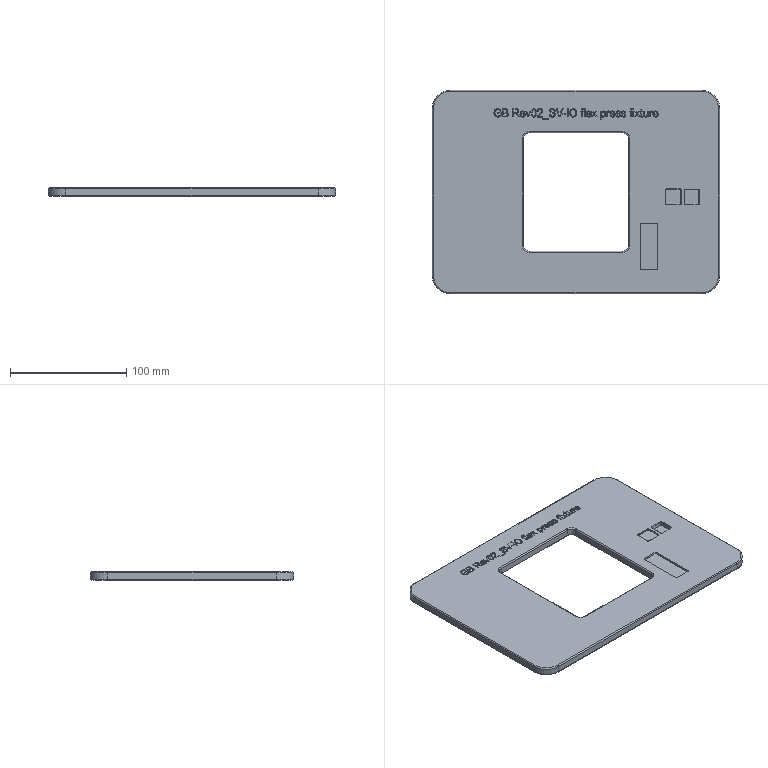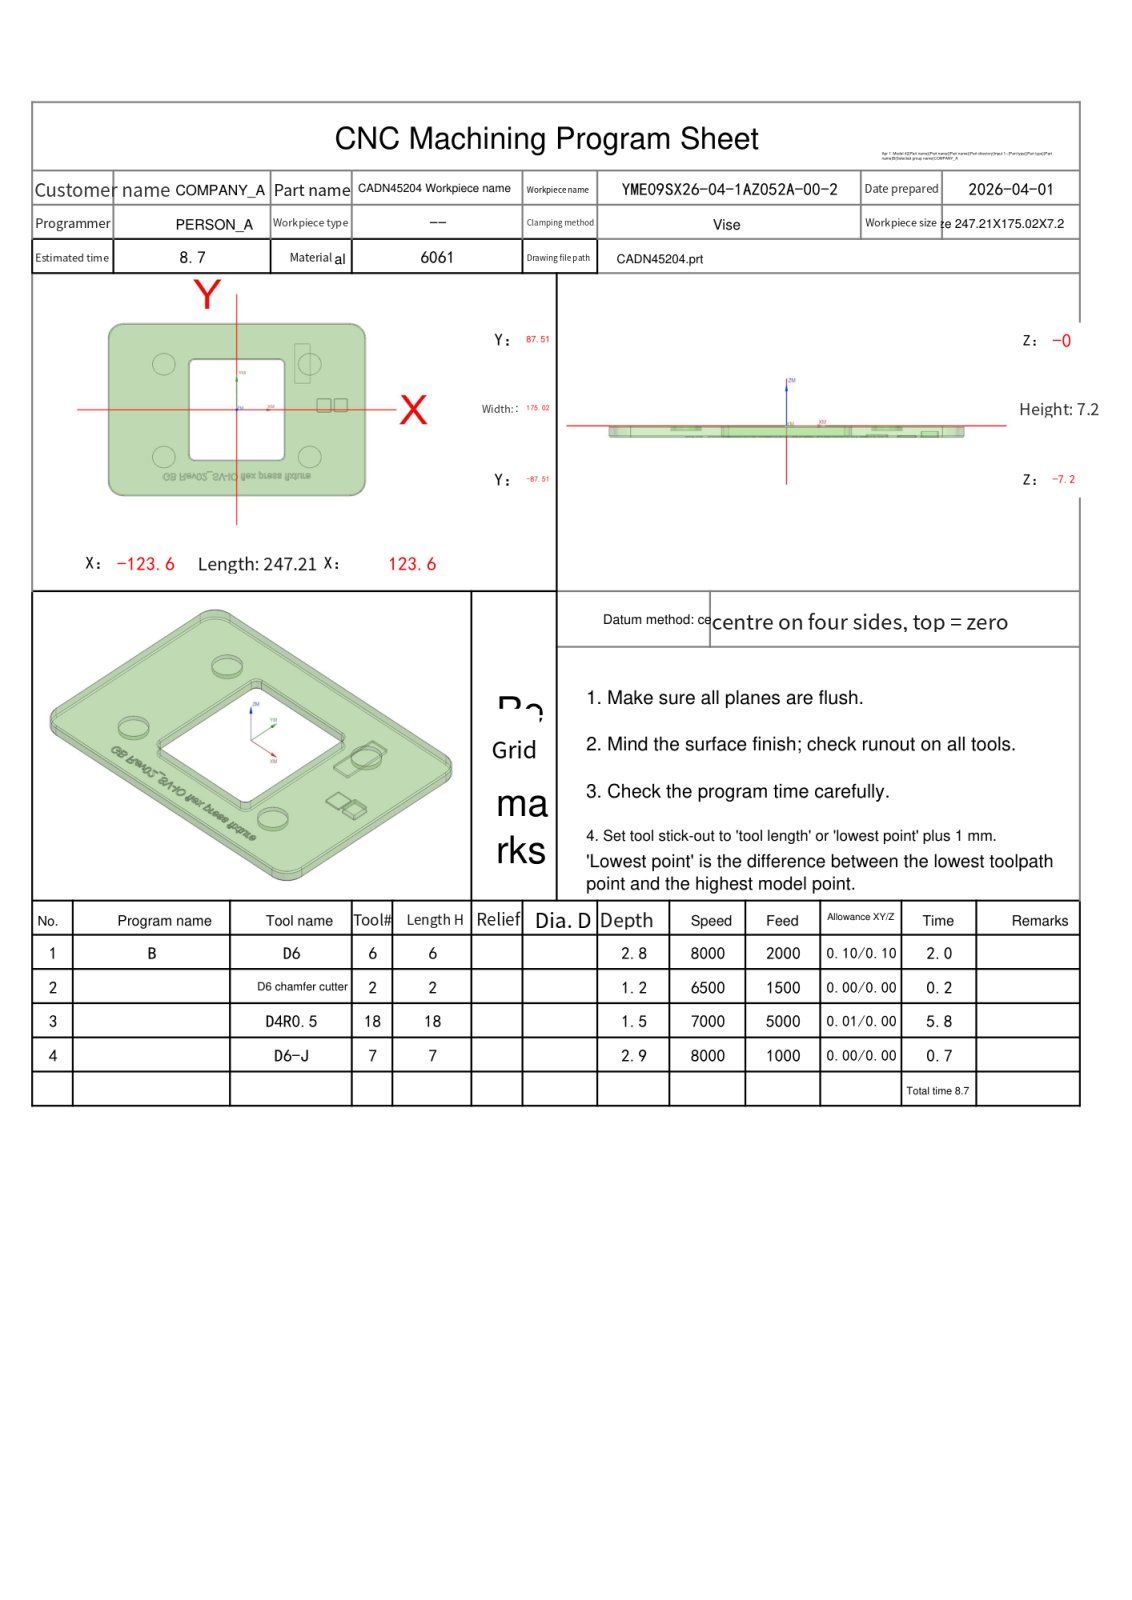NC program | NX | posted by the shop | part box 247.208 x 175.016 x 7.2 mm
Lines 996 to 2593 of 22917:
N3 T18 M06
(D4R0.5  D=4. R=0.5 H=18 ce=0.01 di=0.00)
G00 G90 G54 X18.353 Y-50.167 M03 S7000
G43 H18 Z50.
M08
Z1.5
G01 X40.571 Z.336 F5000.
X41.147 Y-50.101 Z.305
X41.709 Y-49.958 Z.275
X42.246 Y-49.741 Z.244
X42.75 Y-49.455 Z.214
X43.211 Y-49.103 Z.184
X43.621 Y-48.693 Z.153
X43.972 Y-48.232 Z.123
X44.259 Y-47.729 Z.093
X44.476 Y-47.191 Z.062
X44.619 Y-46.629 Z.032
X44.685 Y-46.054 Z.001
Y-45.846 Z-.009
Y45.846
G03 X40.363 Y50.167 I-4.322 J0.0
G01 X-40.359
G03 X-44.681 Y45.846 I0.0 J-4.322
G01 Y-45.846
G03 X-40.359 Y-50.167 I4.322 J0.0
G01 X40.363
G03 X44.685 Y-45.846 I0.0 J4.322
G01 Y-43.852 Z-.01
X44.684 Y-41.859
X44.683 Y-39.866
Y-37.872
X44.681 Y-35.879
Y-33.886
X44.68 Y-31.893
Y-29.899
X44.678 Y-27.906
Y-25.913
X44.677 Y-23.919
Y-21.926
X44.676 Y-19.933 Z-.011
Y-17.94
X44.674 Y-15.946
Y-13.953
X44.673 Y-11.96
Y-9.966
X44.672 Y-7.973
X44.671 Y-5.98
X44.67 Y-3.987
Y-1.993
X44.669 Y0.0
X44.668 Y1.993
Y3.987 Z-.012
X44.667 Y5.98
X44.666 Y7.973
X44.665 Y9.966
Y11.96
X44.664 Y13.953
Y15.946
X44.663 Y17.94
X44.662 Y19.933
X44.661 Y21.926
Y23.919
X44.66 Y25.913 Z-.013
Y27.906
X44.659 Y29.899
X44.658 Y31.893
Y33.886
X44.657 Y35.879
X44.656 Y37.872
Y39.866
X44.655 Y41.859
X44.654 Y43.852
Y45.846
X44.649 Y46.044
X44.636 Y46.241
X44.612 Y46.438
X44.581 Y46.634
X44.539 Y46.828
X44.49 Y47.02
X44.431 Y47.209
X44.364 Y47.395
X44.288 Y47.578
X44.204 Y47.758
X44.111 Y47.933
X44.011 Y48.104
X43.902 Y48.27
X43.787 Y48.431
X43.663 Y48.586
X43.533 Y48.736 Z-.014
X43.396 Y48.879
X43.253 Y49.016
X43.103 Y49.145
X42.948 Y49.269
X42.787 Y49.384
X42.621 Y49.492
X42.45 Y49.593
X42.275 Y49.685
X42.096 Y49.769
X41.913 Y49.845
X41.726 Y49.912
X41.537 Y49.971
X41.345 Y50.02
X41.151 Y50.061
X40.956 Y50.093
X40.759 Y50.116
X40.561 Y50.129
X40.363 Y50.134
X38.441
X36.519 Y50.133
X34.597
X32.675 Y50.132
X30.753
X28.831 Y50.131
X26.909
X24.987 Y50.129
X23.066 Y50.13
X21.144 Y50.128
X19.222 Z-.015
X17.3 Y50.127
X15.378
X13.456 Y50.126
X11.534
X9.612 Y50.125
X7.69
X5.768 Y50.124
X3.846
X1.924 Y50.122
X.002 Y50.123
X-1.92 Y50.121
X-3.842 Z-.016
X-5.764 Y50.12
X-7.686
X-9.608 Y50.119
X-11.53
X-13.452 Y50.118
X-15.374
X-17.296 Y50.116
X-19.218 Y50.117
X-21.14 Y50.115
X-23.062
X-24.984 Y50.114
X-26.906 Z-.017
X-28.828 Y50.113
X-30.75
X-32.672 Y50.112
X-34.594
X-36.515 Y50.111
X-38.437
X-40.359 Y50.11
X-40.556 Y50.105
X-40.753 Y50.092
X-40.949 Y50.069
X-41.143 Y50.037
X-41.336 Y49.996
X-41.526 Y49.947
X-41.714 Y49.889
X-41.9 Y49.822
X-42.082 Y49.746
X-42.26 Y49.662
X-42.434 Y49.57
X-42.604 Y49.471
X-42.769 Y49.363
X-42.929 Y49.248
X-43.083 Y49.126
X-43.232 Y48.996
X-43.374 Y48.86
X-43.51 Y48.718
X-43.639 Y48.569
X-43.762 Y48.415
X-43.877 Y48.255
X-43.984 Y48.09
X-44.084 Y47.92
X-44.176 Y47.746
X-44.259 Y47.567
X-44.335 Y47.386
X-44.401 Y47.2
X-44.46 Y47.012
X-44.509 Y46.822
X-44.55 Y46.629
X-44.581 Y46.434
X-44.604 Y46.239
X-44.617 Y46.042
X-44.622 Y45.846
X-44.621 Y43.852
Y41.859 Z-.018
X-44.62 Y39.866
Y37.872
X-44.619 Y35.879
Y33.886
X-44.618 Y31.893
Y29.899
X-44.617 Y27.906
Y25.913
X-44.616 Y23.919
Y21.926
X-44.615 Y19.933
Y17.94 Z-.019
X-44.614 Y15.946
Y13.953
X-44.613 Y11.96
X-44.612 Y9.966
Y7.973
X-44.611 Y5.98
Y3.987
X-44.61 Y1.993
Y0.0
X-44.609 Y-1.993
Y-3.987 Z-.02
X-44.608 Y-5.98
Y-7.973
X-44.607 Y-9.966
Y-11.96
X-44.606 Y-13.953
Y-15.946
X-44.605 Y-17.94
Y-19.933
X-44.604 Y-21.926
Y-23.919
X-44.603 Y-25.913
Y-27.906 Z-.021
X-44.602 Y-29.899
Y-31.893
X-44.601 Y-33.886
Y-35.879
X-44.6 Y-37.872
Y-39.866
X-44.599 Y-41.859
Y-43.852
X-44.598 Y-45.846
X-44.593 Y-46.041
X-44.579 Y-46.237
X-44.557 Y-46.431
X-44.525 Y-46.624
X-44.485 Y-46.816
X-44.436 Y-47.005
X-44.378 Y-47.192
X-44.311 Y-47.376
X-44.236 Y-47.557
X-44.153 Y-47.734
X-44.062 Y-47.908
X-43.962 Y-48.076
X-43.855 Y-48.24
X-43.741 Y-48.399
X-43.62 Y-48.553
X-43.491 Y-48.7
X-43.356 Y-48.842
X-43.214 Y-48.977
X-43.066 Y-49.106
X-42.913 Y-49.227
X-42.754 Y-49.341
X-42.59 Y-49.448
X-42.421 Y-49.547
X-42.248 Y-49.638 Z-.022
X-42.071 Y-49.722
X-41.89 Y-49.796
X-41.706 Y-49.863
X-41.519 Y-49.921
X-41.329 Y-49.97
X-41.138 Y-50.01
X-40.945 Y-50.042
X-40.75 Y-50.064
X-40.555 Y-50.078
X-40.359 Y-50.082
X-38.437
X-36.515 Y-50.081
X-34.594
X-32.672 Y-50.08
X-30.75
X-28.828 Y-50.079
X-26.906
X-24.984 Y-50.078
X-23.062
X-21.14
X-19.218 Y-50.077
X-17.296 Z-.023
X-15.374 Y-50.076
X-13.452
X-11.53 Y-50.075
X-9.608
X-7.686 Y-50.074
X-5.764
X-3.842 Y-50.073
X-1.92
X.002 Y-50.072
X1.924
X3.846 Y-50.071
X5.768 Z-.024
X7.69 Y-50.07
X9.612
X11.534
X13.456 Y-50.069
X15.378
X17.3
X19.222 Y-50.068
X21.144
X23.066 Y-50.067
X24.987
X26.909 Y-50.066
X28.831 Z-.025
X30.753 Y-50.065
X32.675
X34.597 Y-50.064
X36.519
X38.441
X40.363 Y-50.063
X40.558 Y-50.058
X40.752 Y-50.045
X40.946 Y-50.022
X41.138 Y-49.991
X41.329 Y-49.951
X41.517 Y-49.902
X41.703 Y-49.844
X41.887 Y-49.778
X42.067 Y-49.703
X42.243 Y-49.621
X42.415 Y-49.529
X42.583 Y-49.431
X42.746 Y-49.324
X42.904 Y-49.211
X43.057 Y-49.09
X43.204 Y-48.962
X43.345 Y-48.827
X43.479 Y-48.686
X43.607 Y-48.539
X43.728 Y-48.387
X43.842 Y-48.228
X43.948 Y-48.065
X44.047 Y-47.897
X44.138 Y-47.725
X44.22 Y-47.549
X44.295 Y-47.369
X44.361 Y-47.185
X44.419 Y-46.999
X44.467 Y-46.811
X44.508 Y-46.62
X44.539 Y-46.428
X44.561 Y-46.235
X44.575 Y-46.04
X44.579 Y-45.846
X44.578 Y-43.852
Y-41.859 Z-.026
X44.577 Y-39.866
Y-37.872
X44.576 Y-35.879
X44.575 Y-33.886
Y-31.893
X44.574 Y-29.899
X44.573 Y-27.906
Y-25.913 Z-.027
X44.572 Y-23.919
Y-21.926
X44.571 Y-19.933
X44.57 Y-17.94
Y-15.946
X44.569 Y-13.953
X44.568 Y-11.96
Y-9.966
X44.567 Y-7.973 Z-.028
X44.566 Y-5.98
Y-3.987
X44.565 Y-1.993
Y0.0
X44.564 Y1.993
X44.563 Y3.987
Y5.98
X44.562 Y7.973 Z-.029
X44.561 Y9.966
Y11.96
X44.56 Y13.953
Y15.946
X44.559 Y17.94
X44.558 Y19.933
Y21.926
X44.557 Y23.919 Z-.03
Y25.913
X44.556 Y27.906
X44.555 Y29.899
Y31.893
X44.554 Y33.886
X44.553 Y35.879
Y37.872
X44.552 Y39.866 Z-.031
Y41.859
X44.551 Y43.852
Y45.846
X44.546 Y46.039
X44.533 Y46.232
X44.51 Y46.424
X44.479 Y46.615
X44.439 Y46.804
X44.391 Y46.991
X44.333 Y47.176
X44.268 Y47.358
X44.193 Y47.537
X44.111 Y47.712
X44.021 Y47.883
X43.923 Y48.05
X43.817 Y48.212
X43.704 Y48.369
X43.584 Y48.52
X43.457 Y48.666
X43.324 Y48.806
X43.184 Y48.94
X43.038 Y49.066
X42.886 Y49.186
X42.729 Y49.299
X42.567 Y49.405
X42.4 Y49.503
X42.229 Y49.593
X42.054 Y49.675
X41.875 Y49.749
X41.693 Y49.814
X41.509 Y49.872
X41.322 Y49.92
X41.132 Y49.96
X40.942 Y49.991
X40.749 Y50.014
X40.557 Y50.027
X40.363 Y50.031
X38.441
X36.519 Y50.03
X34.597 Z-.032
X32.675 Y50.029
X30.753
X28.831 Y50.028
X26.909
X24.987 Y50.027
X23.066
X21.144 Y50.026
X19.222 Z-.033
X17.3 Y50.025
X15.378 Y50.024
X13.456
X11.534 Y50.023
X9.612 Y50.022
X7.69
X5.768 Y50.021
X3.846
X1.924 Y50.02 Z-.034
X.002
X-1.92 Y50.019
X-3.842
X-5.764 Y50.018
X-7.686
X-9.608 Y50.017
X-11.53
X-13.452 Y50.016 Z-.035
X-15.374 Y50.015
X-17.296
X-19.218 Y50.014
X-21.14
X-23.062 Y50.013
X-24.984
X-26.906 Y50.012
X-28.828 Y50.011
X-30.75 Z-.036
X-32.672 Y50.01
X-34.594
X-36.515 Y50.009
X-38.437
X-40.359 Y50.008
X-40.552 Y50.004
X-40.744 Y49.991
X-40.935 Y49.969
X-41.124 Y49.937
X-41.312 Y49.898
X-41.499 Y49.849
X-41.682 Y49.792
X-41.863 Y49.727
X-42.041 Y49.653
X-42.215 Y49.571
X-42.385 Y49.482
X-42.551 Y49.384
X-42.712 Y49.279
X-42.868 Y49.167
X-43.018 Y49.048
X-43.163 Y48.921
X-43.302 Y48.789
X-43.435 Y48.649
X-43.561 Y48.504
X-43.681 Y48.354
X-43.793 Y48.198
X-43.898 Y48.036
X-43.995 Y47.871
X-44.085 Y47.701
X-44.167 Y47.527
X-44.24 Y47.349
X-44.305 Y47.168
X-44.362 Y46.984
X-44.41 Y46.798
X-44.45 Y46.61
X-44.481 Y46.42 Z-.037
X-44.503 Y46.23
X-44.516 Y46.038
X-44.521 Y45.846
X-44.52 Y43.852
X-44.519 Y41.859
Y39.866
X-44.518 Y37.872
Y35.879
X-44.517 Y33.886
Y31.893
X-44.516 Y29.899 Z-.038
Y27.906
X-44.515 Y25.913
Y23.919
X-44.514 Y21.926
Y19.933
X-44.513 Y17.94
Y15.946
X-44.512 Y13.953
Y11.96 Z-.039
X-44.511 Y9.966
Y7.973
X-44.51 Y5.98
Y3.987
X-44.509 Y1.993
Y0.0
X-44.508 Y-1.993
Y-3.987 Z-.04
X-44.507 Y-5.98
Y-7.973
X-44.506 Y-9.966
Y-11.96
X-44.505 Y-13.953
Y-15.946
X-44.504 Y-17.94
Y-19.933 Z-.041
X-44.503 Y-21.926
Y-23.919
X-44.502 Y-25.913
Y-27.906
X-44.501 Y-29.899
Y-31.893
X-44.5 Y-33.886
Y-35.879
X-44.499 Y-37.872 Z-.042
Y-39.866
X-44.498 Y-41.859
Y-43.852
X-44.497 Y-45.846
X-44.492 Y-46.037
X-44.479 Y-46.227
X-44.457 Y-46.417
X-44.426 Y-46.606
X-44.387 Y-46.793
X-44.338 Y-46.978
X-44.282 Y-47.16
X-44.217 Y-47.34
X-44.144 Y-47.517
X-44.063 Y-47.689
X-43.974 Y-47.859
X-43.877 Y-48.023
X-43.772 Y-48.183
X-43.661 Y-48.338
X-43.542 Y-48.488
X-43.416 Y-48.632
X-43.284 Y-48.771
X-43.146 Y-48.902
X-43.002 Y-49.028
X-42.852 Y-49.146
X-42.697 Y-49.258
X-42.537 Y-49.362
X-42.372 Y-49.459
X-42.203 Y-49.548
X-42.03 Y-49.629
X-41.854 Y-49.702
X-41.674 Y-49.767
X-41.491 Y-49.824
X-41.306 Y-49.872
X-41.119 Y-49.911
X-40.931 Y-49.942
X-40.741 Y-49.964
X-40.55 Y-49.977
X-40.359 Y-49.981
X-38.437 Z-.043
X-36.515 Y-49.98
X-34.594
X-32.672 Y-49.979
X-30.75
X-28.828 Y-49.978
X-26.906
X-24.984 Y-49.977
X-23.062 Z-.044
X-21.14 Y-49.976
X-19.218
X-17.296
X-15.374
X-13.452 Y-49.975
X-11.53
X-9.608 Y-49.974
X-7.686
X-5.764 Y-49.973 Z-.045
X-3.842
X-1.92 Y-49.972
X.002
X1.924 Y-49.971
X3.846
X5.768 Y-49.97
X7.69
X9.612 Y-49.969 Z-.046
X11.534
X13.456 Y-49.968
X15.378
X17.3 Y-49.967
X19.222
X21.144 Y-49.966
X23.066
X24.987
X26.909 Z-.047
X28.831 Y-49.965
X30.753
X32.675 Y-49.964
X34.597
X36.519 Y-49.963
X38.441
X40.363 Y-49.962
X40.553 Y-49.957
X40.743 Y-49.944
X40.932 Y-49.922
X41.12 Y-49.892
X41.306 Y-49.852
X41.49 Y-49.805
X41.671 Y-49.748
X41.85 Y-49.684
X42.026 Y-49.611
X42.198 Y-49.53
X42.366 Y-49.441
X42.53 Y-49.345 Z-.048
X42.689 Y-49.241
X42.844 Y-49.13
X42.992 Y-49.012
X43.136 Y-48.887
X43.273 Y-48.756
X43.405 Y-48.618
X43.529 Y-48.475
X43.647 Y-48.326
X43.758 Y-48.171
X43.862 Y-48.012
X43.958 Y-47.848
X44.047 Y-47.68
X44.128 Y-47.508
X44.201 Y-47.332
X44.265 Y-47.153
X44.321 Y-46.972
X44.369 Y-46.788
X44.408 Y-46.602
X44.439 Y-46.414
X44.461 Y-46.225
X44.474 Y-46.036
X44.478 Y-45.846
X44.477 Y-43.852
Y-41.859
X44.476 Y-39.866
Y-37.872
X44.475 Y-35.879 Z-.049
X44.474 Y-33.886
Y-31.893
X44.473 Y-29.899
Y-27.906
X44.472 Y-25.913
X44.471 Y-23.919
Y-21.926 Z-.05
X44.47 Y-19.933
Y-17.94
X44.469 Y-15.946
Y-13.953
X44.468 Y-11.96
X44.467 Y-9.966 Z-.051
Y-7.973
X44.466 Y-5.98
Y-3.987
X44.465 Y-1.993
Y0.0
X44.464 Y1.993
X44.463 Y3.987 Z-.052
Y5.98
X44.462 Y7.973
X44.461 Y9.966
Y11.96
X44.46 Y13.953
Y15.946 Z-.053
X44.459 Y17.94
Y19.933
X44.458 Y21.926
Y23.919
X44.457 Y25.913
Y27.906 Z-.054
X44.456 Y29.899
Y31.893
X44.455 Y33.886
Y35.879
X44.454 Y37.872
X44.453 Y39.866
X44.452 Y41.859 Z-.055
Y43.852
X44.451 Y45.846
X44.446 Y46.046
X44.432 Y46.246
X44.407 Y46.445
X44.373 Y46.643
X44.328 Y46.839
X44.275 Y47.032
X44.212 Y47.223
X44.14 Y47.41
X44.058 Y47.593
X43.968 Y47.772
X43.869 Y47.947
X43.762 Y48.116
X43.646 Y48.28
X43.523 Y48.439
X43.392 Y48.59
X43.253 Y48.736
X43.108 Y48.874
X42.956 Y49.005
X42.798 Y49.128
X42.634 Y49.244
X42.464 Y49.351
X42.29 Y49.45
X42.111 Y49.54
X41.927 Y49.621
X41.74 Y49.693
X41.55 Y49.756
X41.356 Y49.81
X41.16 Y49.854
X40.963 Y49.888
X40.764 Y49.912
X40.564 Y49.927
X40.363 Y49.932
X38.441 Z-.056
X36.519 Y49.931
X34.597
X32.675 Y49.93
X30.753
X28.831 Y49.929
X26.909 Y49.928
X24.987 Z-.057
X23.066 Y49.927
X21.144
X19.222 Y49.926
X17.3
X15.378 Y49.925
X13.456 Z-.058
X11.534 Y49.924
X9.612 Y49.923
X7.69
X5.768 Y49.922
X3.846
X1.924 Y49.921
X.002 Z-.059
X-1.92 Y49.92
X-3.842
X-5.764 Y49.919
X-7.686
X-9.608 Y49.918
X-11.53 Y49.917
X-13.452 Z-.06
X-15.374 Y49.916
X-17.296
X-19.218
X-21.14 Y49.915
X-23.062
X-24.984 Y49.914
X-26.906 Z-.061
X-28.828 Y49.913
X-30.75
X-32.672 Y49.912
X-34.594
X-36.515 Y49.911
X-38.437 Z-.062
X-40.359 Y49.91
X-40.559 Y49.905
X-40.758 Y49.89
X-40.956 Y49.866
X-41.152 Y49.832
X-41.347 Y49.788
X-41.539 Y49.735
X-41.729 Y49.672
X-41.915 Y49.6
X-42.097 Y49.519
X-42.275 Y49.429
X-42.449 Y49.331
X-42.617 Y49.224
X-42.78 Y49.11
X-42.937 Y48.987
X-43.088 Y48.856
X-43.233 Y48.719
X-43.37 Y48.574
X-43.5 Y48.423
X-43.623 Y48.266
X-43.738 Y48.103
X-43.845 Y47.934
X-43.943 Y47.761
X-44.032 Y47.583
X-44.113 Y47.4
X-44.185 Y47.214
X-44.247 Y47.025
X-44.301 Y46.833
X-44.344 Y46.638
X-44.378 Y46.442
X-44.403 Y46.244
X-44.417 Y46.045
X-44.422 Y45.846
Y43.852
X-44.421 Y41.859 Z-.063
Y39.866
X-44.42 Y37.872
Y35.879
X-44.419 Y33.886
Y31.893
X-44.418 Y29.899
Y27.906 Z-.064
X-44.417 Y25.913
Y23.919
X-44.416 Y21.926
Y19.933
X-44.415 Y17.94
Y15.946 Z-.065
X-44.414 Y13.953
Y11.96
X-44.413 Y9.966
Y7.973
X-44.412 Y5.98
Y3.987
X-44.411 Y1.993 Z-.066
Y0.0
X-44.41 Y-1.993
Y-3.987
X-44.409 Y-5.98
Y-7.973
X-44.408 Y-9.966 Z-.067
Y-11.96
X-44.407 Y-13.953
Y-15.946
X-44.406 Y-17.94
Y-19.933
X-44.405 Y-21.926
Y-23.919 Z-.068
X-44.404 Y-25.913
Y-27.906
X-44.403 Y-29.899
Y-31.893
X-44.402 Y-33.886
Y-35.879 Z-.069
X-44.401 Y-37.872
Y-39.866
X-44.4 Y-41.859
Y-43.852
X-44.399 Y-45.846
X-44.394 Y-46.044
X-44.379 Y-46.241
X-44.355 Y-46.438
X-44.321 Y-46.634
X-44.277 Y-46.827
X-44.225 Y-47.018
X-44.162 Y-47.206
X-44.091 Y-47.391
X-44.011 Y-47.572
X-43.921 Y-47.749
X-43.824 Y-47.922 Z-.07
X-43.718 Y-48.089
X-43.603 Y-48.251
X-43.481 Y-48.408
X-43.352 Y-48.558
X-43.215 Y-48.701
X-43.072 Y-48.838
X-42.921 Y-48.967
X-42.765 Y-49.089
X-42.603 Y-49.203
X-42.436 Y-49.309
X-42.263 Y-49.407
X-42.086 Y-49.496
X-41.905 Y-49.576
X-41.72 Y-49.648
X-41.532 Y-49.71
X-41.341 Y-49.763
X-41.147 Y-49.806
X-40.952 Y-49.84
X-40.755 Y-49.864
X-40.558 Y-49.879
X-40.359 Y-49.883
X-38.437
X-36.515 Y-49.882
X-34.594
X-32.672 Y-49.881
X-30.75 Y-49.882 Z-.071
X-28.828 Y-49.88
X-26.906 Y-49.881
X-24.984 Y-49.879
X-23.062 Y-49.88
X-21.14 Y-49.879
X-19.218
X-17.296 Y-49.878 Z-.072
X-15.374
X-13.452 Y-49.877
X-11.53
X-9.608 Y-49.876
X-7.686
X-5.764 Y-49.875 Z-.073
X-3.842
X-1.92 Y-49.874
X.002
X1.924 Y-49.873
X3.846
X5.768 Y-49.872
X7.69 Z-.074
X9.612 Y-49.871
X11.534
X13.456 Y-49.87
X15.378
X17.3
X19.222 Y-49.869
X21.144 Z-.075
X23.066 Y-49.868
X24.987
X26.909 Y-49.867
X28.831
X30.753
X32.675 Y-49.866 Z-.076
X34.597
X36.519 Y-49.865
X38.441
X40.363 Y-49.864
X40.56 Y-49.859
X40.757 Y-49.845
X40.953 Y-49.82
X41.147 Y-49.787
X41.34 Y-49.743
X41.53 Y-49.691
X41.717 Y-49.629
X41.901 Y-49.558
X42.081 Y-49.478
X42.257 Y-49.389
X42.429 Y-49.292
X42.595 Y-49.186
X42.757 Y-49.073
X42.912 Y-48.951
X43.061 Y-48.822
X43.204 Y-48.687
X43.34 Y-48.544
X43.469 Y-48.394
X43.59 Y-48.239
X43.704 Y-48.078
X43.809 Y-47.911
X43.906 Y-47.739
X43.995 Y-47.563
X44.075 Y-47.383
X44.146 Y-47.199 Z-.077
X44.208 Y-47.012
X44.26 Y-46.822
X44.303 Y-46.629
X44.337 Y-46.435
X44.361 Y-46.239
X44.375 Y-46.043
X44.38 Y-45.846
Y-43.852
X44.379 Y-41.859
Y-39.866
X44.378 Y-37.872
Y-35.879 Z-.078
X44.377 Y-33.886
Y-31.893
X44.376 Y-29.899
X44.375 Y-27.906
Y-25.913 Z-.079
X44.374 Y-23.919
X44.373 Y-21.926
Y-19.933
X44.372 Y-17.94
Y-15.946
X44.371 Y-13.953 Z-.08
Y-11.96
X44.37 Y-9.966
Y-7.973
X44.369 Y-5.98
Y-3.987 Z-.081
X44.368 Y-1.993
Y0.0
X44.367 Y1.993
Y3.987
X44.365 Y5.98 Z-.082
Y7.973
X44.364 Y9.966
Y11.96
X44.363 Y13.953
Y15.946
X44.362 Y17.94 Z-.083
Y19.933
X44.361 Y21.926
Y23.919
X44.36 Y25.913
Y27.906 Z-.084
X44.359 Y29.899
Y31.893
X44.358 Y33.886
Y35.879
X44.357 Y37.872 Z-.085
Y39.866
X44.356 Y41.859
Y43.852
X44.355 Y45.846
X44.35 Y46.041
X44.335 Y46.237
X44.311 Y46.431
X44.278 Y46.624
X44.235 Y46.815
X44.183 Y47.004
X44.121 Y47.19
X44.05 Y47.373
X43.971 Y47.552 Z-.086
X43.883 Y47.727
X43.786 Y47.897
X43.682 Y48.063
X43.569 Y48.223
X43.448 Y48.377
X43.32 Y48.525
X43.185 Y48.667
X43.043 Y48.802
X42.895 Y48.93
X42.74 Y49.051
X42.58 Y49.163
X42.415 Y49.268
X42.244 Y49.365
X42.069 Y49.453
X41.89 Y49.532
X41.707 Y49.602
X41.521 Y49.664
X41.333 Y49.716
X41.142 Y49.759
X40.949 Y49.792
X40.754 Y49.816
X40.559 Y49.83
X40.363 Y49.835
X38.441
X36.519 Y49.834
X34.597
X32.675 Y49.833 Z-.087
X30.753
X28.831 Y49.832
X26.909
X24.987 Y49.831
X23.066 Z-.088
X21.144 Y49.83
X19.222
X17.3 Y49.829
X15.378
X13.456 Y49.828
X11.534 Z-.089
X9.612 Y49.827
X7.69
X5.768 Y49.826
X3.846
X1.924 Y49.825 Z-.09
X.002
X-1.92 Y49.824
X-3.842
X-5.764 Y49.823
X-7.686 Z-.091
X-9.608 Y49.822
X-11.53
X-13.452 Y49.821
X-15.374
X-17.296 Y49.82
X-19.218 Z-.092
X-21.14 Y49.819
X-23.062
X-24.984 Y49.818
X-26.906
X-28.828 Y49.817 Z-.093
X-30.75
X-32.672 Y49.816
X-34.594
X-36.515 Y49.815
X-38.437
X-40.359 Y49.814 Z-.094
X-40.554 Y49.809
X-40.748 Y49.795
X-40.942 Y49.771
X-41.134 Y49.738
X-41.324 Y49.695
X-41.511 Y49.643
X-41.696 Y49.582
X-41.878 Y49.512
X-42.056 Y49.433
X-42.23 Y49.345
X-42.399 Y49.249
X-42.564 Y49.145
X-42.723 Y49.033
X-42.877 Y48.913
X-43.024 Y48.785
X-43.165 Y48.651
X-43.299 Y48.51
X-43.426 Y48.363
X-43.546 Y48.209
X-43.658 Y48.05
X-43.762 Y47.885
X-43.858 Y47.716
X-43.946 Y47.542
X-44.025 Y47.364
X-44.095 Y47.182
X-44.156 Y46.997
X-44.208 Y46.81
X-44.25 Y46.619
X-44.284 Y46.428
X-44.307 Y46.234
X-44.322 Y46.04
X-44.326 Y45.846
Y43.852
X-44.325 Y41.859 Z-.095
Y39.866
X-44.324 Y37.872
Y35.879
X-44.323 Y33.886
Y31.893 Z-.096
X-44.322 Y29.899
Y27.906
X-44.321 Y25.913
Y23.919
X-44.32 Y21.926
Y19.933 Z-.097
X-44.319 Y17.94
Y15.946
X-44.318 Y13.953
Y11.96
X-44.317 Y9.966 Z-.098
Y7.973
X-44.316 Y5.98
Y3.987
X-44.315 Y1.993
Y0.0 Z-.099
X-44.314 Y-1.993
Y-3.987
X-44.313 Y-5.98
Y-7.973
X-44.312 Y-9.966 Z-.1
Y-11.96
X-44.311 Y-13.953
Y-15.946
X-44.31 Y-17.94
Y-19.933
X-44.309 Y-21.926 Z-.101
Y-23.919
X-44.308 Y-25.913
Y-27.906
X-44.307 Y-29.899
Y-31.893 Z-.102
X-44.306 Y-33.886
Y-35.879
X-44.305 Y-37.872
Y-39.866
X-44.304 Y-41.859 Z-.103
Y-43.852
X-44.303 Y-45.846
X-44.299 Y-46.039
X-44.284 Y-46.232
X-44.261 Y-46.424
X-44.228 Y-46.615
X-44.185 Y-46.804
X-44.133 Y-46.99
X-44.073 Y-47.174
X-44.003 Y-47.355
X-43.924 Y-47.532
X-43.837 Y-47.705
X-43.742 Y-47.873
X-43.638 Y-48.036
X-43.527 Y-48.195
X-43.408 Y-48.347
X-43.281 Y-48.494
X-43.148 Y-48.634
X-43.008 Y-48.767
X-42.861 Y-48.894
X-42.708 Y-49.013
X-42.55 Y-49.124
X-42.387 Y-49.228
X-42.218 Y-49.323
X-42.045 Y-49.41
X-41.868 Y-49.488
X-41.688 Y-49.558
X-41.504 Y-49.619
X-41.317 Y-49.67
X-41.129 Y-49.713
X-40.938 Y-49.746
X-40.746 Y-49.769
X-40.553 Y-49.783 Z-.104
X-40.359 Y-49.788
X-38.437
X-36.515 Y-49.787
X-34.594
X-32.672 Y-49.786
X-30.75
X-28.828 Y-49.785 Z-.105
X-26.906
X-24.984 Y-49.784
X-23.062
X-21.14 Y-49.783
X-19.218 Z-.106
X-17.296 Y-49.782
X-15.374
X-13.452
X-11.53 Y-49.781
X-9.608
X-7.686 Y-49.78 Z-.107
X-5.764
X-3.842 Y-49.779
X-1.92
X.002 Y-49.778
X1.924 Z-.108
X3.846 Y-49.777
X5.768
X7.69
X9.612 Y-49.776
X11.534
X13.456 Y-49.775 Z-.109
X15.378
X17.3 Y-49.774
X19.222
X21.144
X23.066 Y-49.773 Z-.11
X24.987
X26.909 Y-49.772
X28.831
X30.753 Y-49.771
X32.675
X34.597 Y-49.77 Z-.111
X36.519
X38.441 Y-49.769
X40.363
X40.556 Y-49.764
X40.748 Y-49.75
X40.939 Y-49.726
X41.129 Y-49.693
X41.316 Y-49.651
X41.502 Y-49.6
X41.685 Y-49.539
X41.865 Y-49.47
X42.041 Y-49.392
X42.213 Y-49.305
X42.38 Y-49.21
X42.543 Y-49.107
X42.7 Y-48.996
X42.852 Y-48.878
X42.998 Y-48.752
X43.137 Y-48.619
X43.27 Y-48.48 Z-.112
X43.395 Y-48.334
X43.514 Y-48.182
X43.625 Y-48.025
X43.728 Y-47.862
X43.823 Y-47.695
X43.909 Y-47.523
X43.987 Y-47.347
X44.056 Y-47.167
X44.117 Y-46.984
X44.168 Y-46.799
X44.21 Y-46.611
X44.243 Y-46.421
X44.266 Y-46.23
X44.281 Y-46.038
X44.285 Y-45.846
Y-43.852
X44.284 Y-41.859
Y-39.866
X44.283 Y-37.872 Z-.113
Y-35.879
X44.282 Y-33.886
Y-31.893
X44.281 Y-29.899 Z-.114
Y-27.906
X44.28 Y-25.913
X44.279 Y-23.919
Y-21.926
X44.278 Y-19.933 Z-.115
Y-17.94
X44.277 Y-15.946
Y-13.953
X44.276 Y-11.96 Z-.116
X44.275 Y-9.966
Y-7.973
X44.274 Y-5.98
Y-3.987
X44.273 Y-1.993 Z-.117
Y0.0
X44.272 Y1.993
Y3.987
X44.271 Y5.98 Z-.118
Y7.973
X44.27 Y9.966
Y11.96
X44.269 Y13.953
Y15.946 Z-.119
X44.268 Y17.94
X44.267 Y19.933
Y21.926
X44.266 Y23.919 Z-.12
Y25.913
X44.265 Y27.906
Y29.899
X44.264 Y31.893
Y33.886 Z-.121
X44.263 Y35.879
Y37.872
X44.262 Y39.866
Y41.859 Z-.122
X44.261 Y43.852
Y45.846
X44.256 Y46.037
X44.242 Y46.228
X44.218 Y46.417
X44.186 Y46.606
X44.144 Y46.793
X44.093 Y46.977
X44.033 Y47.158
X43.964 Y47.337
X43.886 Y47.512
X43.8 Y47.683
X43.706 Y47.849
X43.603 Y48.011
X43.493 Y48.167
X43.376 Y48.318
X43.251 Y48.462
X43.119 Y48.601
X42.98 Y48.733
X42.835 Y48.858
X42.684 Y48.975
X42.528 Y49.085
X42.366 Y49.188 Z-.123
X42.2 Y49.282
X42.029 Y49.368
X41.854 Y49.445
X41.676 Y49.514
X41.494 Y49.574
X41.31 Y49.625
X41.123 Y49.667
X40.935 Y49.699
X40.745 Y49.723
X40.554 Y49.737
X40.363 Y49.742
X38.441 Y49.741
X36.519
X34.597 Y49.74
X32.675 Z-.124
X30.753 Y49.739
X28.831
X26.909 Y49.738
X24.987
X23.066 Y49.737 Z-.125
X21.144
X19.222 Y49.736
X17.3
X15.378 Y49.735 Z-.126
X13.456
X11.534 Y49.734
X9.612
X7.69 Y49.733
X5.768 Z-.127
X3.846 Y49.732
X1.924
X.002 Y49.731
X-1.92
X-3.842 Y49.73 Z-.128
X-5.764
X-7.686 Y49.729
X-9.608
X-11.53 Y49.728 Z-.129
X-13.452
X-15.374 Y49.727
X-17.296
X-19.218 Y49.726
X-21.14 Z-.13
X-23.062 Y49.725
X-24.984
X-26.906 Y49.724
X-28.828
X-30.75 Y49.723 Z-.131
X-32.672
X-34.594 Y49.722
X-36.515
X-38.437 Y49.721 Z-.132
X-40.359
X-40.55 Y49.716
X-40.739 Y49.702
X-40.928 Y49.679
X-41.115 Y49.646
X-41.301 Y49.605
X-41.484 Y49.554
X-41.665 Y49.494
X-41.842 Y49.425
X-42.016 Y49.349
X-42.186 Y49.263
X-42.352 Y49.169
X-42.512 Y49.067
X-42.668 Y48.958
X-42.817 Y48.841
X-42.962 Y48.717
X-43.099 Y48.585
X-43.23 Y48.448
X-43.354 Y48.303
X-43.471 Y48.154
X-43.581 Y47.998
X-43.683 Y47.837
X-43.776 Y47.672
X-43.862 Y47.502
X-43.939 Y47.328
X-44.007 Y47.151
X-44.067 Y46.97
X-44.117 Y46.787
X-44.159 Y46.601
X-44.192 Y46.414
X-44.215 Y46.225
X-44.229 Y46.036
X-44.233 Y45.846
Y43.852 Z-.133
X-44.232 Y41.859
Y39.866
X-44.231 Y37.872
Y35.879 Z-.134
X-44.23 Y33.886
Y31.893
X-44.229 Y29.899
Y27.906
X-44.228 Y25.913 Z-.135
Y23.919
X-44.227 Y21.926
Y19.933
X-44.226 Y17.94 Z-.136
Y15.946
X-44.225 Y13.953
Y11.96
X-44.224 Y9.966
Y7.973 Z-.137
Y5.98
X-44.223 Y3.987
Y1.993
X-44.222 Y0.0 Z-.138
Y-1.993
X-44.221 Y-3.987
Y-5.98
X-44.22 Y-7.973
Y-9.966 Z-.139
X-44.219 Y-11.96
Y-13.953
X-44.218 Y-15.946
Y-17.94 Z-.14
X-44.217 Y-19.933
Y-21.926
X-44.216 Y-23.919
Y-25.913
Y-27.906 Z-.141
X-44.215 Y-29.899
Y-31.893
X-44.214 Y-33.886
Y-35.879 Z-.142
X-44.213 Y-37.872
Y-39.866
X-44.212 Y-41.859
Y-43.852 Z-.143
X-44.211 Y-45.846
X-44.206 Y-46.035
X-44.192 Y-46.223
X-44.169 Y-46.411
X-44.137 Y-46.597
X-44.095 Y-46.781
X-44.045 Y-46.964
X-43.986 Y-47.143
X-43.917 Y-47.319
X-43.841 Y-47.492
X-43.756 Y-47.661
X-43.663 Y-47.825
X-43.561 Y-47.985
X-43.453 Y-48.14
X-43.336 Y-48.289
X-43.213 Y-48.432
X-43.082 Y-48.569
X-42.945 Y-48.699
X-42.802 Y-48.822
X-42.653 Y-48.939
X-42.499 Y-49.047
X-42.339 Y-49.148
X-42.175 Y-49.241
X-42.006 Y-49.326
X-41.833 Y-49.403
X-41.657 Y-49.471
X-41.477 Y-49.53
X-41.295 Y-49.581
X-41.111 Y-49.622
X-40.924 Y-49.654
X-40.737 Y-49.677
X-40.548 Y-49.691
X-40.359 Y-49.696
X-38.437 Y-49.695 Z-.144
X-36.515
X-34.594
X-32.672 Y-49.694
X-30.75
X-28.828 Y-49.693 Z-.145
X-26.906
X-24.984 Y-49.692
X-23.062
X-21.14 Y-49.691 Z-.146
X-19.218
X-17.296 Y-49.69
X-15.374
X-13.452 Y-49.689
X-11.53 Z-.147
X-9.608 Y-49.688
X-7.686
X-5.764 Y-49.687
X-3.842
X-1.92 Z-.148
X.002 Y-49.686
X1.924
X3.846
X5.768 Y-49.685 Z-.149
X7.69
X9.612 Y-49.684
X11.534
X13.456 Y-49.683
X15.378 Z-.15
X17.3 Y-49.682
X19.222
X21.144 Y-49.681
X23.066 Z-.151
X24.987 Y-49.68
X26.909
X28.831
X30.753 Y-49.679
X32.675 Z-.152
X34.597 Y-49.678
X36.519
X38.441
X40.363 Y-49.677
X40.551 Y-49.672
X40.739 Y-49.658
X40.925 Y-49.635 Z-.153
X41.111 Y-49.603
X41.294 Y-49.562
X41.475 Y-49.512
X41.654 Y-49.453
X41.829 Y-49.385
X42.001 Y-49.309
X42.169 Y-49.224
X42.333 Y-49.131
X42.492 Y-49.031
X42.645 Y-48.922
X42.793 Y-48.807
X42.936 Y-48.684
X43.072 Y-48.554
X43.202 Y-48.418
X43.324 Y-48.276
X43.44 Y-48.127
X43.548 Y-47.974
X43.649 Y-47.815
X43.741 Y-47.651
X43.826 Y-47.483
X43.902 Y-47.311
X43.97 Y-47.136
X44.029 Y-46.957
X44.079 Y-46.776
X44.12 Y-46.593
X44.152 Y-46.408
X44.175 Y-46.221
X44.189 Y-46.034
X44.193 Y-45.846
Y-43.852
X44.192 Y-41.859 Z-.154
Y-39.866
X44.191 Y-37.872
Y-35.879
X44.19 Y-33.886 Z-.155
Y-31.893
X44.189 Y-29.899
Y-27.906
X44.188 Y-25.913 Z-.156
Y-23.919
X44.187 Y-21.926
Y-19.933
X44.186 Y-17.94 Z-.157
Y-15.946
X44.185 Y-13.953
Y-11.96
X44.184 Y-9.966 Z-.158
X44.183 Y-7.973
Y-5.98
X44.182 Y-3.987
Y-1.993 Z-.159
X44.181 Y0.0
Y1.993
X44.18 Y3.987 Z-.16
Y5.98
X44.179 Y7.973
Y9.966
X44.178 Y11.96 Z-.161
Y13.953
X44.177 Y15.946
Y17.94
X44.176 Y19.933 Z-.162
Y21.926
X44.175 Y23.919